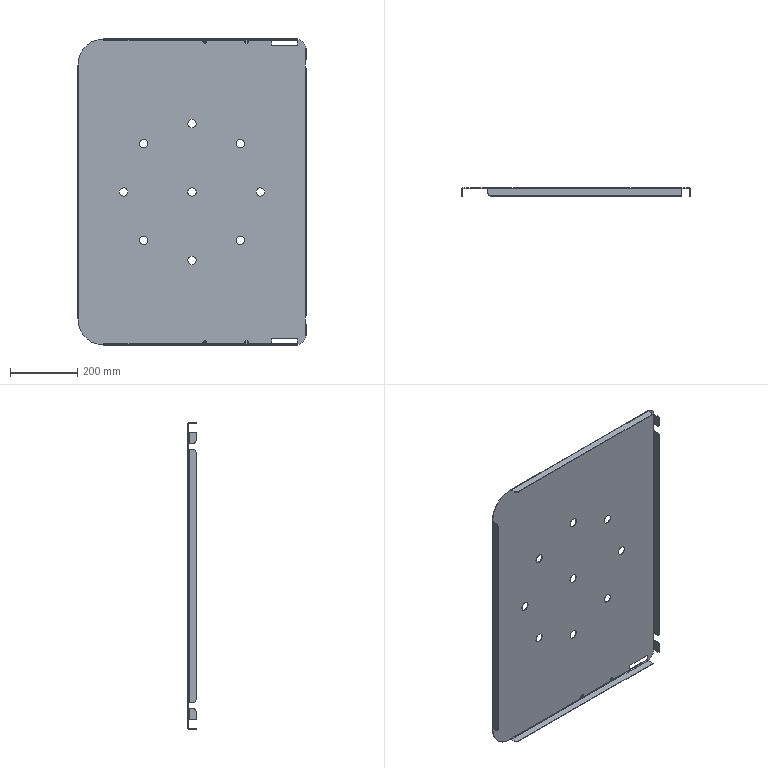Part | NX | features BREP 1 | 1 solid | 156 faces | box 679.907 x 24.003 x 910.285 mm | volume 999074 mm3 | plane 90 | cylinder 58 | spline 8 | commonest cylinder face diameters 25.4 x18 10.998 x8 19.05 x8 1.587 x6 3.175 x6 6.172 x6